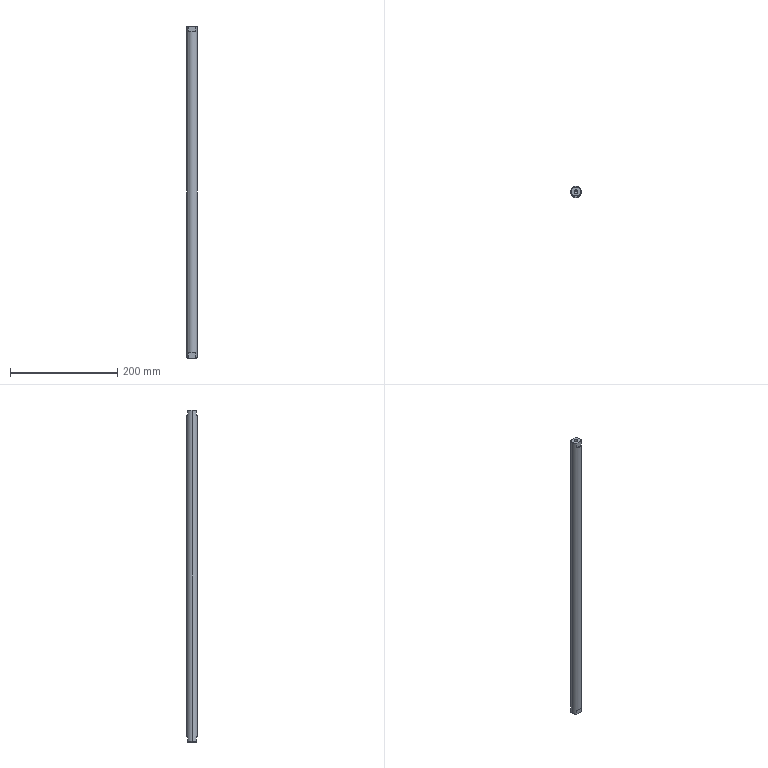Part | STEP file | Ejector rod | 1 solid | 26 faces | box 20 x 20 x 620 mm | volume 192172 mm3 | cone 10 | plane 10 | cylinder 6 | commonest cylinder face diameters 6.8 x4 20 x2